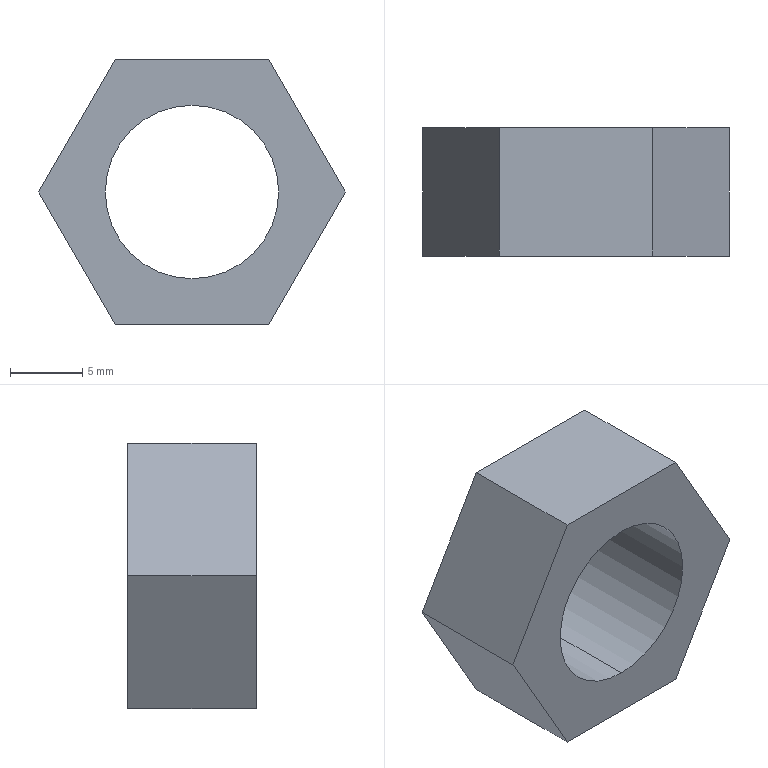Part | SolidWorks | features BaseBody 1 | 1 solid | 10 faces | box 21.246 x 8.9 x 18.4 mm | volume 1603 mm3 | plane 8 | cylinder 2 | commonest cylinder face diameters 12 x2
STEP:
#1=CARTESIAN_POINT('',(0.,0.,-6.));
#2=VERTEX_POINT('',#1);
#3=CARTESIAN_POINT('',(0.,0.,6.));
#4=VERTEX_POINT('',#3);
#5=CARTESIAN_POINT('',(0.,0.,0.));
#6=DIRECTION('',(0.,1.,0.));
#7=DIRECTION('',(0.,0.,1.));
#8=AXIS2_PLACEMENT_3D('',#5,#6,#7);
#9=CIRCLE('',#8,6.);
#10=EDGE_CURVE('',#2,#4,#9,.T.);
#11=ORIENTED_EDGE('',*,*,#10,.F.);
#12=CARTESIAN_POINT('',(0.,8.9,-6.));
#13=VERTEX_POINT('',#12);
#14=CARTESIAN_POINT('',(0.,0.,-6.));
#15=DIRECTION('',(0.,1.,0.));
#16=VECTOR('',#15,1000.);
#17=LINE('',#14,#16);
#18=EDGE_CURVE('',#2,#13,#17,.T.);
#19=ORIENTED_EDGE('',*,*,#18,.T.);
#20=CARTESIAN_POINT('',(0.,8.9,6.));
#21=VERTEX_POINT('',#20);
#22=CARTESIAN_POINT('',(0.,8.9,0.));
#23=DIRECTION('',(0.,-1.,0.));
#24=DIRECTION('',(0.,0.,1.));
#25=AXIS2_PLACEMENT_3D('',#22,#23,#24);
#26=CIRCLE('',#25,6.);
#27=EDGE_CURVE('',#21,#13,#26,.T.);
#28=ORIENTED_EDGE('',*,*,#27,.F.);
#29=CARTESIAN_POINT('',(0.,0.,6.));
#30=DIRECTION('',(0.,1.,0.));
#31=VECTOR('',#30,1000.);
#32=LINE('',#29,#31);
#33=EDGE_CURVE('',#4,#21,#32,.T.);
#34=ORIENTED_EDGE('',*,*,#33,.F.);
#35=EDGE_LOOP('',(#11,#19,#28,#34));
#36=FACE_OUTER_BOUND('',#35,.T.);
#37=CARTESIAN_POINT('',(0.,0.,0.));
#38=DIRECTION('',(0.,1.,0.));
#39=DIRECTION('',(0.,0.,1.));
#40=AXIS2_PLACEMENT_3D('',#37,#38,#39);
#41=CYLINDRICAL_SURFACE('',#40,6.);
#42=ADVANCED_FACE('',(#36),#41,.F.);
#43=CARTESIAN_POINT('',(-10.623,8.9,0.));
#44=VERTEX_POINT('',#43);
#45=CARTESIAN_POINT('',(-5.312,8.9,9.2));
#46=VERTEX_POINT('',#45);
#47=CARTESIAN_POINT('',(-10.623,8.9,0.));
#48=DIRECTION('',(0.5,0.,0.866));
#49=VECTOR('',#48,1000.);
#50=LINE('',#47,#49);
#51=EDGE_CURVE('',#44,#46,#50,.T.);
#52=ORIENTED_EDGE('',*,*,#51,.T.);
#53=CARTESIAN_POINT('',(5.312,8.9,9.2));
#54=VERTEX_POINT('',#53);
#55=CARTESIAN_POINT('',(0.,8.9,9.2));
#56=DIRECTION('',(1.,0.,0.));
#57=VECTOR('',#56,1000.);
#58=LINE('',#55,#57);
#59=EDGE_CURVE('',#46,#54,#58,.T.);
#60=ORIENTED_EDGE('',*,*,#59,.T.);
#61=CARTESIAN_POINT('',(10.623,8.9,0.));
#62=VERTEX_POINT('',#61);
#63=CARTESIAN_POINT('',(5.312,8.9,9.2));
#64=DIRECTION('',(0.5,0.,-0.866));
#65=VECTOR('',#64,1000.);
#66=LINE('',#63,#65);
#67=EDGE_CURVE('',#54,#62,#66,.T.);
#68=ORIENTED_EDGE('',*,*,#67,.T.);
#69=CARTESIAN_POINT('',(5.312,8.9,-9.2));
#70=VERTEX_POINT('',#69);
#71=CARTESIAN_POINT('',(10.623,8.9,0.));
#72=DIRECTION('',(-0.5,0.,-0.866));
#73=VECTOR('',#72,1000.);
#74=LINE('',#71,#73);
#75=EDGE_CURVE('',#62,#70,#74,.T.);
#76=ORIENTED_EDGE('',*,*,#75,.T.);
#77=CARTESIAN_POINT('',(-5.312,8.9,-9.2));
#78=VERTEX_POINT('',#77);
#79=CARTESIAN_POINT('',(0.,8.9,-9.2));
#80=DIRECTION('',(-1.,0.,0.));
#81=VECTOR('',#80,1000.);
#82=LINE('',#79,#81);
#83=EDGE_CURVE('',#70,#78,#82,.T.);
#84=ORIENTED_EDGE('',*,*,#83,.T.);
#85=CARTESIAN_POINT('',(-5.312,8.9,-9.2));
#86=DIRECTION('',(-0.5,0.,0.866));
#87=VECTOR('',#86,1000.);
#88=LINE('',#85,#87);
#89=EDGE_CURVE('',#78,#44,#88,.T.);
#90=ORIENTED_EDGE('',*,*,#89,.T.);
#91=EDGE_LOOP('',(#52,#60,#68,#76,#84,#90));
#92=FACE_OUTER_BOUND('',#91,.T.);
#93=ORIENTED_EDGE('',*,*,#27,.T.);
#94=CARTESIAN_POINT('',(0.,8.9,0.));
#95=DIRECTION('',(0.,-1.,0.));
#96=DIRECTION('',(0.,0.,1.));
#97=AXIS2_PLACEMENT_3D('',#94,#95,#96);
#98=CIRCLE('',#97,6.);
#99=EDGE_CURVE('',#13,#21,#98,.T.);
#100=ORIENTED_EDGE('',*,*,#99,.T.);
#101=EDGE_LOOP('',(#93,#100));
#102=FACE_BOUND('',#101,.T.);
#103=CARTESIAN_POINT('',(0.,8.9,0.));
#104=DIRECTION('',(0.,1.,0.));
#105=DIRECTION('',(0.,0.,1.));
#106=AXIS2_PLACEMENT_3D('',#103,#104,#105);
#107=PLANE('',#106);
#108=ADVANCED_FACE('',(#92,#102),#107,.T.);
#109=CARTESIAN_POINT('',(5.312,0.,9.2));
#110=VERTEX_POINT('',#109);
#111=CARTESIAN_POINT('',(5.312,8.9,9.2));
#112=DIRECTION('',(0.,-1.,0.));
#113=VECTOR('',#112,1000.);
#114=LINE('',#111,#113);
#115=EDGE_CURVE('',#54,#110,#114,.T.);
#116=ORIENTED_EDGE('',*,*,#115,.F.);
#117=ORIENTED_EDGE('',*,*,#59,.F.);
#118=CARTESIAN_POINT('',(-5.312,0.,9.2));
#119=VERTEX_POINT('',#118);
#120=CARTESIAN_POINT('',(-5.312,8.9,9.2));
#121=DIRECTION('',(0.,1.,0.));
#122=VECTOR('',#121,1000.);
#123=LINE('',#120,#122);
#124=EDGE_CURVE('',#119,#46,#123,.T.);
#125=ORIENTED_EDGE('',*,*,#124,.F.);
#126=CARTESIAN_POINT('',(-5.312,0.,9.2));
#127=DIRECTION('',(-1.,0.,0.));
#128=VECTOR('',#127,1000.);
#129=LINE('',#126,#128);
#130=EDGE_CURVE('',#110,#119,#129,.T.);
#131=ORIENTED_EDGE('',*,*,#130,.F.);
#132=EDGE_LOOP('',(#116,#117,#125,#131));
#133=FACE_OUTER_BOUND('',#132,.T.);
#134=CARTESIAN_POINT('',(-5.312,8.9,9.2));
#135=DIRECTION('',(0.,0.,-1.));
#136=DIRECTION('',(-1.,0.,0.));
#137=AXIS2_PLACEMENT_3D('',#134,#135,#136);
#138=PLANE('',#137);
#139=ADVANCED_FACE('',(#133),#138,.F.);
#140=ORIENTED_EDGE('',*,*,#124,.T.);
#141=ORIENTED_EDGE('',*,*,#51,.F.);
#142=CARTESIAN_POINT('',(-10.623,0.,0.));
#143=VERTEX_POINT('',#142);
#144=CARTESIAN_POINT('',(-10.623,8.9,0.));
#145=DIRECTION('',(0.,1.,0.));
#146=VECTOR('',#145,1000.);
#147=LINE('',#144,#146);
#148=EDGE_CURVE('',#143,#44,#147,.T.);
#149=ORIENTED_EDGE('',*,*,#148,.F.);
#150=CARTESIAN_POINT('',(-10.623,0.,0.));
#151=DIRECTION('',(-0.5,0.,-0.866));
#152=VECTOR('',#151,1000.);
#153=LINE('',#150,#152);
#154=EDGE_CURVE('',#119,#143,#153,.T.);
#155=ORIENTED_EDGE('',*,*,#154,.F.);
#156=EDGE_LOOP('',(#140,#141,#149,#155));
#157=FACE_OUTER_BOUND('',#156,.T.);
#158=CARTESIAN_POINT('',(-10.623,8.9,0.));
#159=DIRECTION('',(0.866,0.,-0.5));
#160=DIRECTION('',(-0.5,0.,-0.866));
#161=AXIS2_PLACEMENT_3D('',#158,#159,#160);
#162=PLANE('',#161);
#163=ADVANCED_FACE('',(#157),#162,.F.);
#164=ORIENTED_EDGE('',*,*,#148,.T.);
#165=ORIENTED_EDGE('',*,*,#89,.F.);
#166=CARTESIAN_POINT('',(-5.312,0.,-9.2));
#167=VERTEX_POINT('',#166);
#168=CARTESIAN_POINT('',(-5.312,8.9,-9.2));
#169=DIRECTION('',(0.,1.,0.));
#170=VECTOR('',#169,1000.);
#171=LINE('',#168,#170);
#172=EDGE_CURVE('',#167,#78,#171,.T.);
#173=ORIENTED_EDGE('',*,*,#172,.F.);
#174=CARTESIAN_POINT('',(-5.312,0.,-9.2));
#175=DIRECTION('',(0.5,0.,-0.866));
#176=VECTOR('',#175,1000.);
#177=LINE('',#174,#176);
#178=EDGE_CURVE('',#143,#167,#177,.T.);
#179=ORIENTED_EDGE('',*,*,#178,.F.);
#180=EDGE_LOOP('',(#164,#165,#173,#179));
#181=FACE_OUTER_BOUND('',#180,.T.);
#182=CARTESIAN_POINT('',(-5.312,8.9,-9.2));
#183=DIRECTION('',(0.866,0.,0.5));
#184=DIRECTION('',(0.5,0.,-0.866));
#185=AXIS2_PLACEMENT_3D('',#182,#183,#184);
#186=PLANE('',#185);
#187=ADVANCED_FACE('',(#181),#186,.F.);
#188=ORIENTED_EDGE('',*,*,#172,.T.);
#189=ORIENTED_EDGE('',*,*,#83,.F.);
#190=CARTESIAN_POINT('',(5.312,0.,-9.2));
#191=VERTEX_POINT('',#190);
#192=CARTESIAN_POINT('',(5.312,8.9,-9.2));
#193=DIRECTION('',(0.,1.,0.));
#194=VECTOR('',#193,1000.);
#195=LINE('',#192,#194);
#196=EDGE_CURVE('',#191,#70,#195,.T.);
#197=ORIENTED_EDGE('',*,*,#196,.F.);
#198=CARTESIAN_POINT('',(5.312,0.,-9.2));
#199=DIRECTION('',(1.,0.,0.));
#200=VECTOR('',#199,1000.);
#201=LINE('',#198,#200);
#202=EDGE_CURVE('',#167,#191,#201,.T.);
#203=ORIENTED_EDGE('',*,*,#202,.F.);
#204=EDGE_LOOP('',(#188,#189,#197,#203));
#205=FACE_OUTER_BOUND('',#204,.T.);
#206=CARTESIAN_POINT('',(5.312,8.9,-9.2));
#207=DIRECTION('',(0.,0.,1.));
#208=DIRECTION('',(1.,0.,0.));
#209=AXIS2_PLACEMENT_3D('',#206,#207,#208);
#210=PLANE('',#209);
#211=ADVANCED_FACE('',(#205),#210,.F.);
#212=ORIENTED_EDGE('',*,*,#196,.T.);
#213=ORIENTED_EDGE('',*,*,#75,.F.);
#214=CARTESIAN_POINT('',(10.623,0.,0.));
#215=VERTEX_POINT('',#214);
#216=CARTESIAN_POINT('',(10.623,8.9,0.));
#217=DIRECTION('',(0.,1.,0.));
#218=VECTOR('',#217,1000.);
#219=LINE('',#216,#218);
#220=EDGE_CURVE('',#215,#62,#219,.T.);
#221=ORIENTED_EDGE('',*,*,#220,.F.);
#222=CARTESIAN_POINT('',(10.623,0.,0.));
#223=DIRECTION('',(0.5,0.,0.866));
#224=VECTOR('',#223,1000.);
#225=LINE('',#222,#224);
#226=EDGE_CURVE('',#191,#215,#225,.T.);
#227=ORIENTED_EDGE('',*,*,#226,.F.);
#228=EDGE_LOOP('',(#212,#213,#221,#227));
#229=FACE_OUTER_BOUND('',#228,.T.);
#230=CARTESIAN_POINT('',(10.623,8.9,0.));
#231=DIRECTION('',(-0.866,0.,0.5));
#232=DIRECTION('',(0.5,0.,0.866));
#233=AXIS2_PLACEMENT_3D('',#230,#231,#232);
#234=PLANE('',#233);
#235=ADVANCED_FACE('',(#229),#234,.F.);
#236=ORIENTED_EDGE('',*,*,#220,.T.);
#237=ORIENTED_EDGE('',*,*,#67,.F.);
#238=ORIENTED_EDGE('',*,*,#115,.T.);
#239=CARTESIAN_POINT('',(5.312,0.,9.2));
#240=DIRECTION('',(-0.5,0.,0.866));
#241=VECTOR('',#240,1000.);
#242=LINE('',#239,#241);
#243=EDGE_CURVE('',#215,#110,#242,.T.);
#244=ORIENTED_EDGE('',*,*,#243,.F.);
#245=EDGE_LOOP('',(#236,#237,#238,#244));
#246=FACE_OUTER_BOUND('',#245,.T.);
#247=CARTESIAN_POINT('',(5.312,8.9,9.2));
#248=DIRECTION('',(-0.866,0.,-0.5));
#249=DIRECTION('',(-0.5,0.,0.866));
#250=AXIS2_PLACEMENT_3D('',#247,#248,#249);
#251=PLANE('',#250);
#252=ADVANCED_FACE('',(#246),#251,.F.);
#253=ORIENTED_EDGE('',*,*,#18,.F.);
#254=CARTESIAN_POINT('',(0.,0.,0.));
#255=DIRECTION('',(0.,1.,0.));
#256=DIRECTION('',(0.,0.,1.));
#257=AXIS2_PLACEMENT_3D('',#254,#255,#256);
#258=CIRCLE('',#257,6.);
#259=EDGE_CURVE('',#4,#2,#258,.T.);
#260=ORIENTED_EDGE('',*,*,#259,.F.);
#261=ORIENTED_EDGE('',*,*,#33,.T.);
#262=ORIENTED_EDGE('',*,*,#99,.F.);
#263=EDGE_LOOP('',(#253,#260,#261,#262));
#264=FACE_OUTER_BOUND('',#263,.T.);
#265=CARTESIAN_POINT('',(0.,0.,0.));
#266=DIRECTION('',(0.,1.,0.));
#267=DIRECTION('',(0.,0.,1.));
#268=AXIS2_PLACEMENT_3D('',#265,#266,#267);
#269=CYLINDRICAL_SURFACE('',#268,6.);
#270=ADVANCED_FACE('',(#264),#269,.F.);
#271=ORIENTED_EDGE('',*,*,#130,.T.);
#272=ORIENTED_EDGE('',*,*,#154,.T.);
#273=ORIENTED_EDGE('',*,*,#178,.T.);
#274=ORIENTED_EDGE('',*,*,#202,.T.);
#275=ORIENTED_EDGE('',*,*,#226,.T.);
#276=ORIENTED_EDGE('',*,*,#243,.T.);
#277=EDGE_LOOP('',(#271,#272,#273,#274,#275,#276));
#278=FACE_OUTER_BOUND('',#277,.T.);
#279=ORIENTED_EDGE('',*,*,#259,.T.);
#280=ORIENTED_EDGE('',*,*,#10,.T.);
#281=EDGE_LOOP('',(#279,#280));
#282=FACE_BOUND('',#281,.T.);
#283=CARTESIAN_POINT('',(0.,0.,0.));
#284=DIRECTION('',(0.,1.,0.));
#285=DIRECTION('',(0.,0.,1.));
#286=AXIS2_PLACEMENT_3D('',#283,#284,#285);
#287=PLANE('',#286);
#288=ADVANCED_FACE('',(#278,#282),#287,.F.);
#289=CLOSED_SHELL('',(#42,#108,#139,#163,#187,#211,#235,#252,#270,#288));
#290=MANIFOLD_SOLID_BREP('',#289);
#291=CARTESIAN_POINT('',(0.,0.,0.));
#292=DIRECTION('',(0.,0.,1.));
#293=DIRECTION('',(1.,0.,0.));
#294=AXIS2_PLACEMENT_3D('',#291,#292,#293);
#295=(LENGTH_UNIT()NAMED_UNIT(*)SI_UNIT(.MILLI.,.METRE.));
#296=UNCERTAINTY_MEASURE_WITH_UNIT(LENGTH_MEASURE(0.00001),#295,'','');
#297=(NAMED_UNIT(*)PLANE_ANGLE_UNIT()SI_UNIT($,.RADIAN.));
#298=(NAMED_UNIT(*)SI_UNIT($,.STERADIAN.)SOLID_ANGLE_UNIT());
#299=(GEOMETRIC_REPRESENTATION_CONTEXT(3)GLOBAL_UNCERTAINTY_ASSIGNED_CONTEXT((#296))GLOBAL_UNIT_ASSIGNED_CONTEXT((#295,#297,#298))REPRESENTATION_CONTEXT('',''));
#300=ADVANCED_BREP_SHAPE_REPRESENTATION('',(#290,#294),#299);